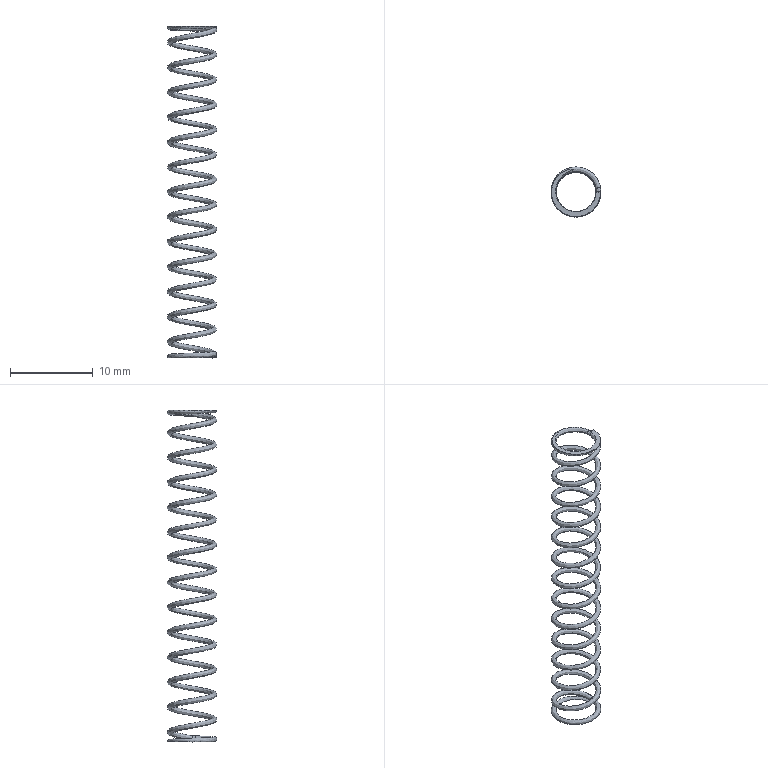Part | STEP file | 1 solid | 9 faces | volume 70.891 mm3 | spline 5 | plane 4